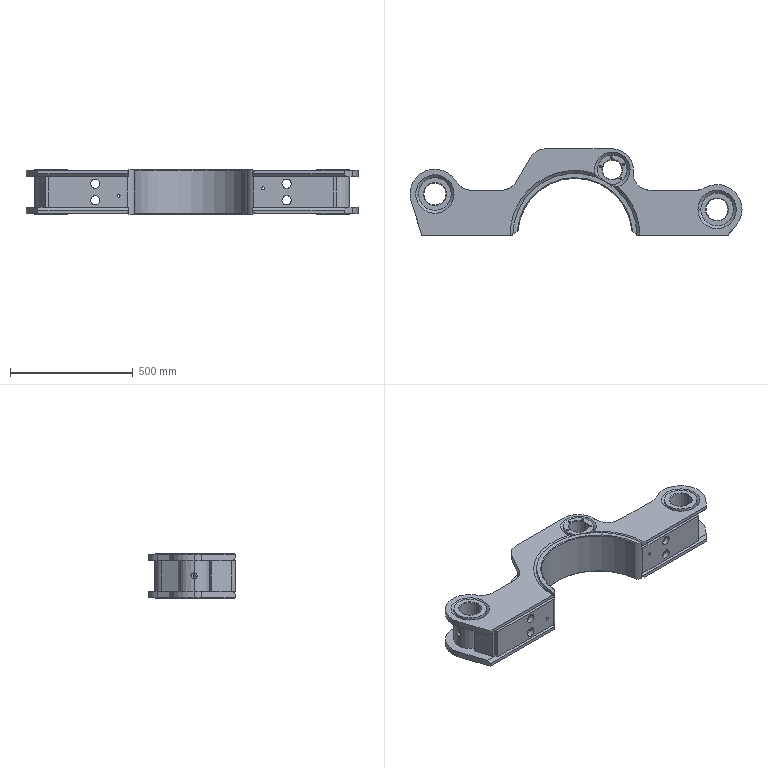Part | SolidWorks | features AEMSimFeature 1, MirrorCompFeat 1, ReferencePattern 1 | 12 solids | 269 faces | box 1354 x 352.3 x 180 mm | volume 22821153 mm3 | cylinder 115 | plane 114 | cone 40 | commonest cylinder face diameters 38 x24 8.5 x14 133 x12 140 x12 121 x9 203 x6